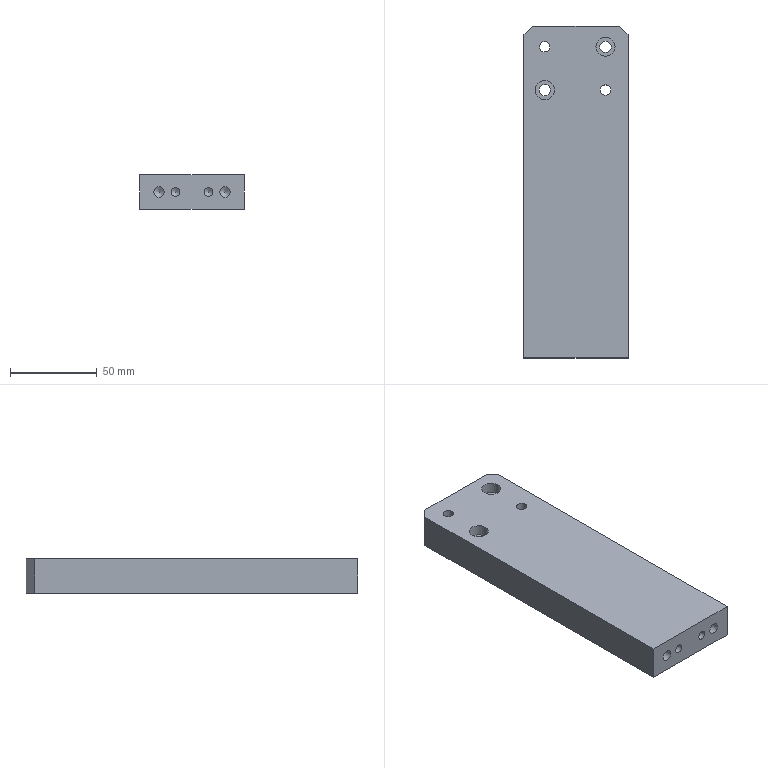Part | NX | features BREP 1 | 1 solid | 24 faces | box 60 x 191.5 x 20 mm | volume 224701 mm3 | plane 10 | cylinder 10 | cone 4 | commonest cylinder face diameters 6 x4 5 x2 6.6 x2 11 x2
STEP:
#1=CARTESIAN_POINT('',(-25.,95.75,0.));
#2=VERTEX_POINT('',#1);
#3=CARTESIAN_POINT('',(-30.,90.75,0.));
#4=VERTEX_POINT('',#3);
#5=CARTESIAN_POINT('',(-25.,95.75,0.));
#6=DIRECTION('',(-0.7071,-0.7071,0.));
#7=VECTOR('',#6,1000.);
#8=LINE('',#5,#7);
#9=EDGE_CURVE('',#2,#4,#8,.T.);
#10=ORIENTED_EDGE('',*,*,#9,.F.);
#11=CARTESIAN_POINT('',(25.,95.75,0.));
#12=VERTEX_POINT('',#11);
#13=CARTESIAN_POINT('',(0.,95.75,0.));
#14=DIRECTION('',(-1.,0.,0.));
#15=VECTOR('',#14,1000.);
#16=LINE('',#13,#15);
#17=EDGE_CURVE('',#12,#2,#16,.T.);
#18=ORIENTED_EDGE('',*,*,#17,.F.);
#19=CARTESIAN_POINT('',(30.,90.75,0.));
#20=VERTEX_POINT('',#19);
#21=CARTESIAN_POINT('',(30.,90.75,0.));
#22=DIRECTION('',(-0.7071,0.7071,0.));
#23=VECTOR('',#22,1000.);
#24=LINE('',#21,#23);
#25=EDGE_CURVE('',#20,#12,#24,.T.);
#26=ORIENTED_EDGE('',*,*,#25,.F.);
#27=CARTESIAN_POINT('',(30.,-95.75,0.));
#28=VERTEX_POINT('',#27);
#29=CARTESIAN_POINT('',(30.,0.,0.));
#30=DIRECTION('',(0.,1.,0.));
#31=VECTOR('',#30,1000.);
#32=LINE('',#29,#31);
#33=EDGE_CURVE('',#28,#20,#32,.T.);
#34=ORIENTED_EDGE('',*,*,#33,.F.);
#35=CARTESIAN_POINT('',(-30.,-95.75,0.));
#36=VERTEX_POINT('',#35);
#37=CARTESIAN_POINT('',(0.,-95.75,0.));
#38=DIRECTION('',(1.,0.,0.));
#39=VECTOR('',#38,1000.);
#40=LINE('',#37,#39);
#41=EDGE_CURVE('',#36,#28,#40,.T.);
#42=ORIENTED_EDGE('',*,*,#41,.F.);
#43=CARTESIAN_POINT('',(-30.,0.,0.));
#44=DIRECTION('',(0.,-1.,0.));
#45=VECTOR('',#44,1000.);
#46=LINE('',#43,#45);
#47=EDGE_CURVE('',#4,#36,#46,.T.);
#48=ORIENTED_EDGE('',*,*,#47,.F.);
#49=EDGE_LOOP('',(#10,#18,#26,#34,#42,#48));
#50=FACE_BOUND('',#49,.T.);
#51=CARTESIAN_POINT('',(-14.7,58.75,0.));
#52=VERTEX_POINT('',#51);
#53=CARTESIAN_POINT('',(-18.,58.75,0.));
#54=DIRECTION('',(0.,0.,-1.));
#55=DIRECTION('',(1.,0.,0.));
#56=AXIS2_PLACEMENT_3D('',#53,#54,#55);
#57=CIRCLE('',#56,3.3);
#58=EDGE_CURVE('',#52,#52,#57,.T.);
#59=ORIENTED_EDGE('',*,*,#58,.F.);
#60=EDGE_LOOP('',(#59));
#61=FACE_BOUND('',#60,.T.);
#62=CARTESIAN_POINT('',(20.3,83.75,0.));
#63=VERTEX_POINT('',#62);
#64=CARTESIAN_POINT('',(17.,83.75,0.));
#65=DIRECTION('',(0.,0.,-1.));
#66=DIRECTION('',(1.,0.,0.));
#67=AXIS2_PLACEMENT_3D('',#64,#65,#66);
#68=CIRCLE('',#67,3.3);
#69=EDGE_CURVE('',#63,#63,#68,.T.);
#70=ORIENTED_EDGE('',*,*,#69,.F.);
#71=EDGE_LOOP('',(#70));
#72=FACE_BOUND('',#71,.T.);
#73=CARTESIAN_POINT('',(-21.,83.75,0.));
#74=VERTEX_POINT('',#73);
#75=CARTESIAN_POINT('',(-18.,83.75,0.));
#76=DIRECTION('',(0.,0.,-1.));
#77=DIRECTION('',(-1.,0.,0.));
#78=AXIS2_PLACEMENT_3D('',#75,#76,#77);
#79=CIRCLE('',#78,3.);
#80=EDGE_CURVE('',#74,#74,#79,.T.);
#81=ORIENTED_EDGE('',*,*,#80,.F.);
#82=EDGE_LOOP('',(#81));
#83=FACE_BOUND('',#82,.T.);
#84=CARTESIAN_POINT('',(14.,58.75,0.));
#85=VERTEX_POINT('',#84);
#86=CARTESIAN_POINT('',(17.,58.75,0.));
#87=DIRECTION('',(0.,0.,-1.));
#88=DIRECTION('',(-1.,0.,0.));
#89=AXIS2_PLACEMENT_3D('',#86,#87,#88);
#90=CIRCLE('',#89,3.);
#91=EDGE_CURVE('',#85,#85,#90,.T.);
#92=ORIENTED_EDGE('',*,*,#91,.F.);
#93=EDGE_LOOP('',(#92));
#94=FACE_BOUND('',#93,.T.);
#95=CARTESIAN_POINT('',(0.,0.,0.));
#96=DIRECTION('',(0.,0.,1.));
#97=DIRECTION('',(-1.,0.,0.));
#98=AXIS2_PLACEMENT_3D('',#95,#96,#97);
#99=PLANE('',#98);
#100=ADVANCED_FACE('',(#50,#61,#72,#83,#94),#99,.F.);
#101=CARTESIAN_POINT('',(-30.,90.75,20.));
#102=VERTEX_POINT('',#101);
#103=CARTESIAN_POINT('',(-30.,90.75,20.));
#104=DIRECTION('',(0.,0.,1.));
#105=VECTOR('',#104,1000.);
#106=LINE('',#103,#105);
#107=EDGE_CURVE('',#4,#102,#106,.T.);
#108=ORIENTED_EDGE('',*,*,#107,.F.);
#109=ORIENTED_EDGE('',*,*,#47,.T.);
#110=CARTESIAN_POINT('',(-30.,-95.75,20.));
#111=VERTEX_POINT('',#110);
#112=CARTESIAN_POINT('',(-30.,-95.75,20.));
#113=DIRECTION('',(0.,0.,-1.));
#114=VECTOR('',#113,1000.);
#115=LINE('',#112,#114);
#116=EDGE_CURVE('',#111,#36,#115,.T.);
#117=ORIENTED_EDGE('',*,*,#116,.F.);
#118=CARTESIAN_POINT('',(-30.,95.75,20.));
#119=DIRECTION('',(0.,-1.,0.));
#120=VECTOR('',#119,1000.);
#121=LINE('',#118,#120);
#122=EDGE_CURVE('',#102,#111,#121,.T.);
#123=ORIENTED_EDGE('',*,*,#122,.F.);
#124=EDGE_LOOP('',(#108,#109,#117,#123));
#125=FACE_BOUND('',#124,.T.);
#126=CARTESIAN_POINT('',(-30.,95.75,20.));
#127=DIRECTION('',(1.,0.,0.));
#128=DIRECTION('',(0.,-1.,0.));
#129=AXIS2_PLACEMENT_3D('',#126,#127,#128);
#130=PLANE('',#129);
#131=ADVANCED_FACE('',(#125),#130,.F.);
#132=CARTESIAN_POINT('',(-25.,95.75,20.));
#133=VERTEX_POINT('',#132);
#134=CARTESIAN_POINT('',(-25.,95.75,20.));
#135=DIRECTION('',(0.,0.,1.));
#136=VECTOR('',#135,1000.);
#137=LINE('',#134,#136);
#138=EDGE_CURVE('',#2,#133,#137,.T.);
#139=ORIENTED_EDGE('',*,*,#138,.F.);
#140=ORIENTED_EDGE('',*,*,#9,.T.);
#141=ORIENTED_EDGE('',*,*,#107,.T.);
#142=CARTESIAN_POINT('',(-30.,90.75,20.));
#143=DIRECTION('',(-0.7071,-0.7071,0.));
#144=VECTOR('',#143,1000.);
#145=LINE('',#142,#144);
#146=EDGE_CURVE('',#133,#102,#145,.T.);
#147=ORIENTED_EDGE('',*,*,#146,.F.);
#148=EDGE_LOOP('',(#139,#140,#141,#147));
#149=FACE_BOUND('',#148,.T.);
#150=CARTESIAN_POINT('',(-30.,90.75,20.));
#151=DIRECTION('',(0.7071,-0.7071,0.));
#152=DIRECTION('',(-0.7071,-0.7071,0.));
#153=AXIS2_PLACEMENT_3D('',#150,#151,#152);
#154=PLANE('',#153);
#155=ADVANCED_FACE('',(#149),#154,.F.);
#156=ORIENTED_EDGE('',*,*,#138,.T.);
#157=CARTESIAN_POINT('',(25.,95.75,20.));
#158=VERTEX_POINT('',#157);
#159=CARTESIAN_POINT('',(-30.,95.75,20.));
#160=DIRECTION('',(-1.,0.,0.));
#161=VECTOR('',#160,1000.);
#162=LINE('',#159,#161);
#163=EDGE_CURVE('',#158,#133,#162,.T.);
#164=ORIENTED_EDGE('',*,*,#163,.F.);
#165=CARTESIAN_POINT('',(25.,95.75,20.));
#166=DIRECTION('',(0.,0.,1.));
#167=VECTOR('',#166,1000.);
#168=LINE('',#165,#167);
#169=EDGE_CURVE('',#12,#158,#168,.T.);
#170=ORIENTED_EDGE('',*,*,#169,.F.);
#171=ORIENTED_EDGE('',*,*,#17,.T.);
#172=EDGE_LOOP('',(#156,#164,#170,#171));
#173=FACE_BOUND('',#172,.T.);
#174=CARTESIAN_POINT('',(-30.,95.75,20.));
#175=DIRECTION('',(0.,-1.,0.));
#176=DIRECTION('',(0.,0.,1.));
#177=AXIS2_PLACEMENT_3D('',#174,#175,#176);
#178=PLANE('',#177);
#179=ADVANCED_FACE('',(#173),#178,.F.);
#180=CARTESIAN_POINT('',(30.,90.75,20.));
#181=VERTEX_POINT('',#180);
#182=CARTESIAN_POINT('',(30.,90.75,20.));
#183=DIRECTION('',(0.,0.,1.));
#184=VECTOR('',#183,1000.);
#185=LINE('',#182,#184);
#186=EDGE_CURVE('',#20,#181,#185,.T.);
#187=ORIENTED_EDGE('',*,*,#186,.F.);
#188=ORIENTED_EDGE('',*,*,#25,.T.);
#189=ORIENTED_EDGE('',*,*,#169,.T.);
#190=CARTESIAN_POINT('',(25.,95.75,20.));
#191=DIRECTION('',(-0.7071,0.7071,0.));
#192=VECTOR('',#191,1000.);
#193=LINE('',#190,#192);
#194=EDGE_CURVE('',#181,#158,#193,.T.);
#195=ORIENTED_EDGE('',*,*,#194,.F.);
#196=EDGE_LOOP('',(#187,#188,#189,#195));
#197=FACE_BOUND('',#196,.T.);
#198=CARTESIAN_POINT('',(25.,95.75,20.));
#199=DIRECTION('',(-0.7071,-0.7071,0.));
#200=DIRECTION('',(-0.7071,0.7071,0.));
#201=AXIS2_PLACEMENT_3D('',#198,#199,#200);
#202=PLANE('',#201);
#203=ADVANCED_FACE('',(#197),#202,.F.);
#204=ORIENTED_EDGE('',*,*,#186,.T.);
#205=CARTESIAN_POINT('',(30.,-95.75,20.));
#206=VERTEX_POINT('',#205);
#207=CARTESIAN_POINT('',(30.,95.75,20.));
#208=DIRECTION('',(0.,1.,0.));
#209=VECTOR('',#208,1000.);
#210=LINE('',#207,#209);
#211=EDGE_CURVE('',#206,#181,#210,.T.);
#212=ORIENTED_EDGE('',*,*,#211,.F.);
#213=CARTESIAN_POINT('',(30.,-95.75,20.));
#214=DIRECTION('',(0.,0.,1.));
#215=VECTOR('',#214,1000.);
#216=LINE('',#213,#215);
#217=EDGE_CURVE('',#28,#206,#216,.T.);
#218=ORIENTED_EDGE('',*,*,#217,.F.);
#219=ORIENTED_EDGE('',*,*,#33,.T.);
#220=EDGE_LOOP('',(#204,#212,#218,#219));
#221=FACE_BOUND('',#220,.T.);
#222=CARTESIAN_POINT('',(30.,95.75,20.));
#223=DIRECTION('',(-1.,0.,0.));
#224=DIRECTION('',(0.,1.,0.));
#225=AXIS2_PLACEMENT_3D('',#222,#223,#224);
#226=PLANE('',#225);
#227=ADVANCED_FACE('',(#221),#226,.F.);
#228=ORIENTED_EDGE('',*,*,#217,.T.);
#229=CARTESIAN_POINT('',(-30.,-95.75,20.));
#230=DIRECTION('',(1.,0.,0.));
#231=VECTOR('',#230,1000.);
#232=LINE('',#229,#231);
#233=EDGE_CURVE('',#111,#206,#232,.T.);
#234=ORIENTED_EDGE('',*,*,#233,.F.);
#235=ORIENTED_EDGE('',*,*,#116,.T.);
#236=ORIENTED_EDGE('',*,*,#41,.T.);
#237=EDGE_LOOP('',(#228,#234,#235,#236));
#238=FACE_BOUND('',#237,.T.);
#239=CARTESIAN_POINT('',(-19.,-95.75,7.));
#240=VERTEX_POINT('',#239);
#241=CARTESIAN_POINT('',(-19.,-95.75,10.));
#242=DIRECTION('',(0.,-1.,0.));
#243=DIRECTION('',(0.,0.,-1.));
#244=AXIS2_PLACEMENT_3D('',#241,#242,#243);
#245=CIRCLE('',#244,3.);
#246=EDGE_CURVE('',#240,#240,#245,.T.);
#247=ORIENTED_EDGE('',*,*,#246,.F.);
#248=EDGE_LOOP('',(#247));
#249=FACE_BOUND('',#248,.T.);
#250=CARTESIAN_POINT('',(19.,-95.75,7.));
#251=VERTEX_POINT('',#250);
#252=CARTESIAN_POINT('',(19.,-95.75,10.));
#253=DIRECTION('',(0.,-1.,0.));
#254=DIRECTION('',(0.,0.,-1.));
#255=AXIS2_PLACEMENT_3D('',#252,#253,#254);
#256=CIRCLE('',#255,3.);
#257=EDGE_CURVE('',#251,#251,#256,.T.);
#258=ORIENTED_EDGE('',*,*,#257,.F.);
#259=EDGE_LOOP('',(#258));
#260=FACE_BOUND('',#259,.T.);
#261=CARTESIAN_POINT('',(-9.5,-95.75,7.5));
#262=VERTEX_POINT('',#261);
#263=CARTESIAN_POINT('',(-9.5,-95.75,10.));
#264=DIRECTION('',(0.,-1.,0.));
#265=DIRECTION('',(0.,0.,-1.));
#266=AXIS2_PLACEMENT_3D('',#263,#264,#265);
#267=CIRCLE('',#266,2.5);
#268=EDGE_CURVE('',#262,#262,#267,.T.);
#269=ORIENTED_EDGE('',*,*,#268,.F.);
#270=EDGE_LOOP('',(#269));
#271=FACE_BOUND('',#270,.T.);
#272=CARTESIAN_POINT('',(9.5,-95.75,7.5));
#273=VERTEX_POINT('',#272);
#274=CARTESIAN_POINT('',(9.5,-95.75,10.));
#275=DIRECTION('',(0.,-1.,0.));
#276=DIRECTION('',(0.,0.,-1.));
#277=AXIS2_PLACEMENT_3D('',#274,#275,#276);
#278=CIRCLE('',#277,2.5);
#279=EDGE_CURVE('',#273,#273,#278,.T.);
#280=ORIENTED_EDGE('',*,*,#279,.F.);
#281=EDGE_LOOP('',(#280));
#282=FACE_BOUND('',#281,.T.);
#283=CARTESIAN_POINT('',(-30.,-95.75,20.));
#284=DIRECTION('',(0.,1.,0.));
#285=DIRECTION('',(0.,0.,-1.));
#286=AXIS2_PLACEMENT_3D('',#283,#284,#285);
#287=PLANE('',#286);
#288=ADVANCED_FACE('',(#238,#249,#260,#271,#282),#287,.F.);
#289=ORIENTED_EDGE('',*,*,#58,.T.);
#290=EDGE_LOOP('',(#289));
#291=FACE_BOUND('',#290,.T.);
#292=CARTESIAN_POINT('',(-14.7,58.75,13.6));
#293=VERTEX_POINT('',#292);
#294=CARTESIAN_POINT('',(-18.,58.75,13.6));
#295=DIRECTION('',(0.,0.,-1.));
#296=DIRECTION('',(1.,0.,0.));
#297=AXIS2_PLACEMENT_3D('',#294,#295,#296);
#298=CIRCLE('',#297,3.3);
#299=EDGE_CURVE('',#293,#293,#298,.T.);
#300=ORIENTED_EDGE('',*,*,#299,.F.);
#301=EDGE_LOOP('',(#300));
#302=FACE_BOUND('',#301,.T.);
#303=CARTESIAN_POINT('',(-18.,58.75,20.));
#304=DIRECTION('',(0.,0.,1.));
#305=DIRECTION('',(-1.,0.,0.));
#306=AXIS2_PLACEMENT_3D('',#303,#304,#305);
#307=CYLINDRICAL_SURFACE('',#306,3.3);
#308=ADVANCED_FACE('',(#291,#302),#307,.F.);
#309=ORIENTED_EDGE('',*,*,#69,.T.);
#310=EDGE_LOOP('',(#309));
#311=FACE_BOUND('',#310,.T.);
#312=CARTESIAN_POINT('',(20.3,83.75,13.6));
#313=VERTEX_POINT('',#312);
#314=CARTESIAN_POINT('',(17.,83.75,13.6));
#315=DIRECTION('',(0.,0.,-1.));
#316=DIRECTION('',(1.,0.,0.));
#317=AXIS2_PLACEMENT_3D('',#314,#315,#316);
#318=CIRCLE('',#317,3.3);
#319=EDGE_CURVE('',#313,#313,#318,.T.);
#320=ORIENTED_EDGE('',*,*,#319,.F.);
#321=EDGE_LOOP('',(#320));
#322=FACE_BOUND('',#321,.T.);
#323=CARTESIAN_POINT('',(17.,83.75,20.));
#324=DIRECTION('',(0.,0.,1.));
#325=DIRECTION('',(-1.,0.,0.));
#326=AXIS2_PLACEMENT_3D('',#323,#324,#325);
#327=CYLINDRICAL_SURFACE('',#326,3.3);
#328=ADVANCED_FACE('',(#311,#322),#327,.F.);
#329=CARTESIAN_POINT('',(-21.,83.75,20.));
#330=VERTEX_POINT('',#329);
#331=CARTESIAN_POINT('',(-18.,83.75,20.));
#332=DIRECTION('',(0.,0.,-1.));
#333=DIRECTION('',(-1.,0.,0.));
#334=AXIS2_PLACEMENT_3D('',#331,#332,#333);
#335=CIRCLE('',#334,3.);
#336=EDGE_CURVE('',#330,#330,#335,.T.);
#337=ORIENTED_EDGE('',*,*,#336,.F.);
#338=EDGE_LOOP('',(#337));
#339=FACE_BOUND('',#338,.T.);
#340=ORIENTED_EDGE('',*,*,#80,.T.);
#341=EDGE_LOOP('',(#340));
#342=FACE_BOUND('',#341,.T.);
#343=CARTESIAN_POINT('',(-18.,83.75,0.));
#344=DIRECTION('',(0.,0.,-1.));
#345=DIRECTION('',(1.,0.,0.));
#346=AXIS2_PLACEMENT_3D('',#343,#344,#345);
#347=CYLINDRICAL_SURFACE('',#346,3.);
#348=ADVANCED_FACE('',(#339,#342),#347,.F.);
#349=CARTESIAN_POINT('',(14.,58.75,20.));
#350=VERTEX_POINT('',#349);
#351=CARTESIAN_POINT('',(17.,58.75,20.));
#352=DIRECTION('',(0.,0.,-1.));
#353=DIRECTION('',(-1.,0.,0.));
#354=AXIS2_PLACEMENT_3D('',#351,#352,#353);
#355=CIRCLE('',#354,3.);
#356=EDGE_CURVE('',#350,#350,#355,.T.);
#357=ORIENTED_EDGE('',*,*,#356,.F.);
#358=EDGE_LOOP('',(#357));
#359=FACE_BOUND('',#358,.T.);
#360=ORIENTED_EDGE('',*,*,#91,.T.);
#361=EDGE_LOOP('',(#360));
#362=FACE_BOUND('',#361,.T.);
#363=CARTESIAN_POINT('',(17.,58.75,0.));
#364=DIRECTION('',(0.,0.,-1.));
#365=DIRECTION('',(1.,0.,0.));
#366=AXIS2_PLACEMENT_3D('',#363,#364,#365);
#367=CYLINDRICAL_SURFACE('',#366,3.);
#368=ADVANCED_FACE('',(#359,#362),#367,.F.);
#369=ORIENTED_EDGE('',*,*,#211,.T.);
#370=ORIENTED_EDGE('',*,*,#194,.T.);
#371=ORIENTED_EDGE('',*,*,#163,.T.);
#372=ORIENTED_EDGE('',*,*,#146,.T.);
#373=ORIENTED_EDGE('',*,*,#122,.T.);
#374=ORIENTED_EDGE('',*,*,#233,.T.);
#375=EDGE_LOOP('',(#369,#370,#371,#372,#373,#374));
#376=FACE_BOUND('',#375,.T.);
#377=CARTESIAN_POINT('',(-12.5,58.75,20.));
#378=VERTEX_POINT('',#377);
#379=CARTESIAN_POINT('',(-18.,58.75,20.));
#380=DIRECTION('',(0.,0.,-1.));
#381=DIRECTION('',(1.,0.,0.));
#382=AXIS2_PLACEMENT_3D('',#379,#380,#381);
#383=CIRCLE('',#382,5.5);
#384=EDGE_CURVE('',#378,#378,#383,.T.);
#385=ORIENTED_EDGE('',*,*,#384,.T.);
#386=EDGE_LOOP('',(#385));
#387=FACE_BOUND('',#386,.T.);
#388=CARTESIAN_POINT('',(22.5,83.75,20.));
#389=VERTEX_POINT('',#388);
#390=CARTESIAN_POINT('',(17.,83.75,20.));
#391=DIRECTION('',(0.,0.,-1.));
#392=DIRECTION('',(1.,0.,0.));
#393=AXIS2_PLACEMENT_3D('',#390,#391,#392);
#394=CIRCLE('',#393,5.5);
#395=EDGE_CURVE('',#389,#389,#394,.T.);
#396=ORIENTED_EDGE('',*,*,#395,.T.);
#397=EDGE_LOOP('',(#396));
#398=FACE_BOUND('',#397,.T.);
#399=ORIENTED_EDGE('',*,*,#336,.T.);
#400=EDGE_LOOP('',(#399));
#401=FACE_BOUND('',#400,.T.);
#402=ORIENTED_EDGE('',*,*,#356,.T.);
#403=EDGE_LOOP('',(#402));
#404=FACE_BOUND('',#403,.T.);
#405=CARTESIAN_POINT('',(0.,0.,20.));
#406=DIRECTION('',(0.,0.,1.));
#407=DIRECTION('',(-1.,0.,0.));
#408=AXIS2_PLACEMENT_3D('',#405,#406,#407);
#409=PLANE('',#408);
#410=ADVANCED_FACE('',(#376,#387,#398,#401,#404),#409,.T.);
#411=CARTESIAN_POINT('',(-19.,-83.75,7.));
#412=VERTEX_POINT('',#411);
#413=CARTESIAN_POINT('',(-19.,-83.75,10.));
#414=DIRECTION('',(0.,-1.,0.));
#415=DIRECTION('',(0.,0.,-1.));
#416=AXIS2_PLACEMENT_3D('',#413,#414,#415);
#417=CIRCLE('',#416,3.);
#418=EDGE_CURVE('',#412,#412,#417,.T.);
#419=ORIENTED_EDGE('',*,*,#418,.F.);
#420=EDGE_LOOP('',(#419));
#421=FACE_BOUND('',#420,.T.);
#422=ORIENTED_EDGE('',*,*,#246,.T.);
#423=EDGE_LOOP('',(#422));
#424=FACE_BOUND('',#423,.T.);
#425=CARTESIAN_POINT('',(-19.,-95.75,10.));
#426=DIRECTION('',(0.,-1.,0.));
#427=DIRECTION('',(0.,0.,1.));
#428=AXIS2_PLACEMENT_3D('',#425,#426,#427);
#429=CYLINDRICAL_SURFACE('',#428,3.);
#430=ADVANCED_FACE('',(#421,#424),#429,.F.);
#431=CARTESIAN_POINT('',(19.,-83.75,7.));
#432=VERTEX_POINT('',#431);
#433=CARTESIAN_POINT('',(19.,-83.75,10.));
#434=DIRECTION('',(0.,-1.,0.));
#435=DIRECTION('',(0.,0.,-1.));
#436=AXIS2_PLACEMENT_3D('',#433,#434,#435);
#437=CIRCLE('',#436,3.);
#438=EDGE_CURVE('',#432,#432,#437,.T.);
#439=ORIENTED_EDGE('',*,*,#438,.F.);
#440=EDGE_LOOP('',(#439));
#441=FACE_BOUND('',#440,.T.);
#442=ORIENTED_EDGE('',*,*,#257,.T.);
#443=EDGE_LOOP('',(#442));
#444=FACE_BOUND('',#443,.T.);
#445=CARTESIAN_POINT('',(19.,-95.75,10.));
#446=DIRECTION('',(0.,-1.,0.));
#447=DIRECTION('',(0.,0.,1.));
#448=AXIS2_PLACEMENT_3D('',#445,#446,#447);
#449=CYLINDRICAL_SURFACE('',#448,3.);
#450=ADVANCED_FACE('',(#441,#444),#449,.F.);
#451=CARTESIAN_POINT('',(-9.5,-80.75,7.5));
#452=VERTEX_POINT('',#451);
#453=CARTESIAN_POINT('',(-9.5,-80.75,10.));
#454=DIRECTION('',(0.,-1.,0.));
#455=DIRECTION('',(0.,0.,-1.));
#456=AXIS2_PLACEMENT_3D('',#453,#454,#455);
#457=CIRCLE('',#456,2.5);
#458=EDGE_CURVE('',#452,#452,#457,.T.);
#459=ORIENTED_EDGE('',*,*,#458,.F.);
#460=EDGE_LOOP('',(#459));
#461=FACE_BOUND('',#460,.T.);
#462=ORIENTED_EDGE('',*,*,#268,.T.);
#463=EDGE_LOOP('',(#462));
#464=FACE_BOUND('',#463,.T.);
#465=CARTESIAN_POINT('',(-9.5,-95.75,10.));
#466=DIRECTION('',(0.,-1.,0.));
#467=DIRECTION('',(0.,0.,1.));
#468=AXIS2_PLACEMENT_3D('',#465,#466,#467);
#469=CYLINDRICAL_SURFACE('',#468,2.5);
#470=ADVANCED_FACE('',(#461,#464),#469,.F.);
#471=CARTESIAN_POINT('',(9.5,-80.75,7.5));
#472=VERTEX_POINT('',#471);
#473=CARTESIAN_POINT('',(9.5,-80.75,10.));
#474=DIRECTION('',(0.,-1.,0.));
#475=DIRECTION('',(0.,0.,-1.));
#476=AXIS2_PLACEMENT_3D('',#473,#474,#475);
#477=CIRCLE('',#476,2.5);
#478=EDGE_CURVE('',#472,#472,#477,.T.);
#479=ORIENTED_EDGE('',*,*,#478,.F.);
#480=EDGE_LOOP('',(#479));
#481=FACE_BOUND('',#480,.T.);
#482=ORIENTED_EDGE('',*,*,#279,.T.);
#483=EDGE_LOOP('',(#482));
#484=FACE_BOUND('',#483,.T.);
#485=CARTESIAN_POINT('',(9.5,-95.75,10.));
#486=DIRECTION('',(0.,-1.,0.));
#487=DIRECTION('',(0.,0.,1.));
#488=AXIS2_PLACEMENT_3D('',#485,#486,#487);
#489=CYLINDRICAL_SURFACE('',#488,2.5);
#490=ADVANCED_FACE('',(#481,#484),#489,.F.);
#491=CARTESIAN_POINT('',(-12.5,58.75,13.6));
#492=VERTEX_POINT('',#491);
#493=CARTESIAN_POINT('',(-18.,58.75,13.6));
#494=DIRECTION('',(0.,0.,-1.));
#495=DIRECTION('',(1.,0.,0.));
#496=AXIS2_PLACEMENT_3D('',#493,#494,#495);
#497=CIRCLE('',#496,5.5);
#498=EDGE_CURVE('',#492,#492,#497,.T.);
#499=ORIENTED_EDGE('',*,*,#498,.F.);
#500=EDGE_LOOP('',(#499));
#501=FACE_BOUND('',#500,.T.);
#502=ORIENTED_EDGE('',*,*,#299,.T.);
#503=EDGE_LOOP('',(#502));
#504=FACE_BOUND('',#503,.T.);
#505=CARTESIAN_POINT('',(-14.7,58.75,13.6));
#506=DIRECTION('',(0.,0.,-1.));
#507=DIRECTION('',(1.,0.,0.));
#508=AXIS2_PLACEMENT_3D('',#505,#506,#507);
#509=PLANE('',#508);
#510=ADVANCED_FACE('',(#501,#504),#509,.F.);
#511=CARTESIAN_POINT('',(22.5,83.75,13.6));
#512=VERTEX_POINT('',#511);
#513=CARTESIAN_POINT('',(17.,83.75,13.6));
#514=DIRECTION('',(0.,0.,-1.));
#515=DIRECTION('',(1.,0.,0.));
#516=AXIS2_PLACEMENT_3D('',#513,#514,#515);
#517=CIRCLE('',#516,5.5);
#518=EDGE_CURVE('',#512,#512,#517,.T.);
#519=ORIENTED_EDGE('',*,*,#518,.F.);
#520=EDGE_LOOP('',(#519));
#521=FACE_BOUND('',#520,.T.);
#522=ORIENTED_EDGE('',*,*,#319,.T.);
#523=EDGE_LOOP('',(#522));
#524=FACE_BOUND('',#523,.T.);
#525=CARTESIAN_POINT('',(20.3,83.75,13.6));
#526=DIRECTION('',(0.,0.,-1.));
#527=DIRECTION('',(1.,0.,0.));
#528=AXIS2_PLACEMENT_3D('',#525,#526,#527);
#529=PLANE('',#528);
#530=ADVANCED_FACE('',(#521,#524),#529,.F.);
#531=ORIENTED_EDGE('',*,*,#384,.F.);
#532=EDGE_LOOP('',(#531));
#533=FACE_BOUND('',#532,.T.);
#534=ORIENTED_EDGE('',*,*,#498,.T.);
#535=EDGE_LOOP('',(#534));
#536=FACE_BOUND('',#535,.T.);
#537=CARTESIAN_POINT('',(-18.,58.75,20.));
#538=DIRECTION('',(0.,0.,1.));
#539=DIRECTION('',(-1.,0.,0.));
#540=AXIS2_PLACEMENT_3D('',#537,#538,#539);
#541=CYLINDRICAL_SURFACE('',#540,5.5);
#542=ADVANCED_FACE('',(#533,#536),#541,.F.);
#543=ORIENTED_EDGE('',*,*,#395,.F.);
#544=EDGE_LOOP('',(#543));
#545=FACE_BOUND('',#544,.T.);
#546=ORIENTED_EDGE('',*,*,#518,.T.);
#547=EDGE_LOOP('',(#546));
#548=FACE_BOUND('',#547,.T.);
#549=CARTESIAN_POINT('',(17.,83.75,20.));
#550=DIRECTION('',(0.,0.,1.));
#551=DIRECTION('',(-1.,0.,0.));
#552=AXIS2_PLACEMENT_3D('',#549,#550,#551);
#553=CYLINDRICAL_SURFACE('',#552,5.5);
#554=ADVANCED_FACE('',(#545,#548),#553,.F.);
#555=CARTESIAN_POINT('',(-19.,-81.947,10.));
#556=VERTEX_POINT('',#555);
#557=VERTEX_LOOP('',#556);
#558=FACE_BOUND('',#557,.T.);
#559=ORIENTED_EDGE('',*,*,#418,.T.);
#560=EDGE_LOOP('',(#559));
#561=FACE_BOUND('',#560,.T.);
#562=CARTESIAN_POINT('',(-19.,-83.75,10.));
#563=DIRECTION('',(0.,-1.,0.));
#564=DIRECTION('',(0.,0.,1.));
#565=AXIS2_PLACEMENT_3D('',#562,#563,#564);
#566=CONICAL_SURFACE('',#565,3.,1.03);
#567=ADVANCED_FACE('',(#558,#561),#566,.F.);
#568=CARTESIAN_POINT('',(19.,-81.947,10.));
#569=VERTEX_POINT('',#568);
#570=VERTEX_LOOP('',#569);
#571=FACE_BOUND('',#570,.T.);
#572=ORIENTED_EDGE('',*,*,#438,.T.);
#573=EDGE_LOOP('',(#572));
#574=FACE_BOUND('',#573,.T.);
#575=CARTESIAN_POINT('',(19.,-83.75,10.));
#576=DIRECTION('',(0.,-1.,0.));
#577=DIRECTION('',(0.,0.,1.));
#578=AXIS2_PLACEMENT_3D('',#575,#576,#577);
#579=CONICAL_SURFACE('',#578,3.,1.03);
#580=ADVANCED_FACE('',(#571,#574),#579,.F.);
#581=CARTESIAN_POINT('',(-9.5,-79.248,10.));
#582=VERTEX_POINT('',#581);
#583=VERTEX_LOOP('',#582);
#584=FACE_BOUND('',#583,.T.);
#585=ORIENTED_EDGE('',*,*,#458,.T.);
#586=EDGE_LOOP('',(#585));
#587=FACE_BOUND('',#586,.T.);
#588=CARTESIAN_POINT('',(-9.5,-80.75,10.));
#589=DIRECTION('',(0.,-1.,0.));
#590=DIRECTION('',(0.,0.,1.));
#591=AXIS2_PLACEMENT_3D('',#588,#589,#590);
#592=CONICAL_SURFACE('',#591,2.5,1.03);
#593=ADVANCED_FACE('',(#584,#587),#592,.F.);
#594=CARTESIAN_POINT('',(9.5,-79.248,10.));
#595=VERTEX_POINT('',#594);
#596=VERTEX_LOOP('',#595);
#597=FACE_BOUND('',#596,.T.);
#598=ORIENTED_EDGE('',*,*,#478,.T.);
#599=EDGE_LOOP('',(#598));
#600=FACE_BOUND('',#599,.T.);
#601=CARTESIAN_POINT('',(9.5,-80.75,10.));
#602=DIRECTION('',(0.,-1.,0.));
#603=DIRECTION('',(0.,0.,1.));
#604=AXIS2_PLACEMENT_3D('',#601,#602,#603);
#605=CONICAL_SURFACE('',#604,2.5,1.03);
#606=ADVANCED_FACE('',(#597,#600),#605,.F.);
#607=CLOSED_SHELL('',(#100,#131,#155,#179,#203,#227,#288,#308,#328,#348,#368,#410,#430,#450,#470,#490,#510,#530,#542,#554,#567,#580,#593,#606));
#608=MANIFOLD_SOLID_BREP('',#607);
#609=(LENGTH_UNIT()NAMED_UNIT(*)SI_UNIT(.MILLI.,.METRE.));
#610=UNCERTAINTY_MEASURE_WITH_UNIT(LENGTH_MEASURE(0.00001),#609,'','');
#611=(NAMED_UNIT(*)PLANE_ANGLE_UNIT()SI_UNIT($,.RADIAN.));
#612=(NAMED_UNIT(*)SI_UNIT($,.STERADIAN.)SOLID_ANGLE_UNIT());
#613=(GEOMETRIC_REPRESENTATION_CONTEXT(3)GLOBAL_UNCERTAINTY_ASSIGNED_CONTEXT((#610))GLOBAL_UNIT_ASSIGNED_CONTEXT((#609,#611,#612))REPRESENTATION_CONTEXT('',''));
#614=ADVANCED_BREP_SHAPE_REPRESENTATION('',(#608),#613);